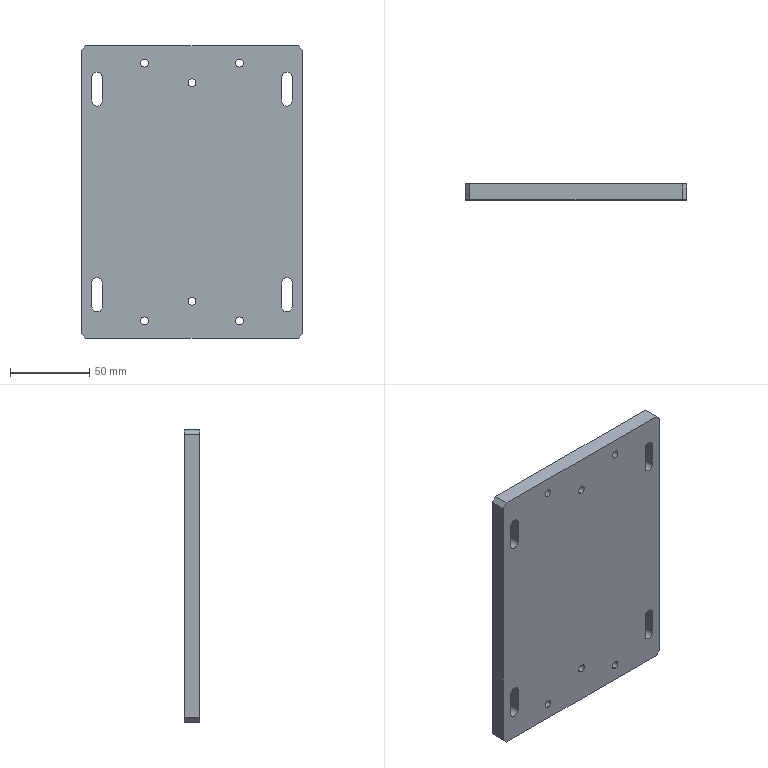Part | SolidWorks | features BaseBody 1 | 1 solid | 42 faces | box 140 x 10 x 185 mm | volume 252313 mm3 | cylinder 24 | plane 18 | commonest cylinder face diameters 5 x12 6.6 x12
STEP:
#1=CARTESIAN_POINT('',(0.,0.,-71.5));
#2=VERTEX_POINT('',#1);
#3=CARTESIAN_POINT('',(0.,10.,-71.5));
#4=VERTEX_POINT('',#3);
#5=CARTESIAN_POINT('',(0.,10.,-71.5));
#6=DIRECTION('',(0.,1.,0.));
#7=VECTOR('',#6,1000.);
#8=LINE('',#5,#7);
#9=EDGE_CURVE('',#2,#4,#8,.T.);
#10=ORIENTED_EDGE('',*,*,#9,.F.);
#11=CARTESIAN_POINT('',(0.,0.,-66.5));
#12=VERTEX_POINT('',#11);
#13=CARTESIAN_POINT('',(0.,0.,-69.));
#14=DIRECTION('',(0.,1.,0.));
#15=DIRECTION('',(0.,0.,1.));
#16=AXIS2_PLACEMENT_3D('',#13,#14,#15);
#17=CIRCLE('',#16,2.5);
#18=EDGE_CURVE('',#12,#2,#17,.T.);
#19=ORIENTED_EDGE('',*,*,#18,.F.);
#20=CARTESIAN_POINT('',(0.,10.,-66.5));
#21=VERTEX_POINT('',#20);
#22=CARTESIAN_POINT('',(0.,10.,-66.5));
#23=DIRECTION('',(0.,1.,0.));
#24=VECTOR('',#23,1000.);
#25=LINE('',#22,#24);
#26=EDGE_CURVE('',#12,#21,#25,.T.);
#27=ORIENTED_EDGE('',*,*,#26,.T.);
#28=CARTESIAN_POINT('',(0.,10.,-69.));
#29=DIRECTION('',(0.,1.,0.));
#30=DIRECTION('',(0.,0.,1.));
#31=AXIS2_PLACEMENT_3D('',#28,#29,#30);
#32=CIRCLE('',#31,2.5);
#33=EDGE_CURVE('',#21,#4,#32,.T.);
#34=ORIENTED_EDGE('',*,*,#33,.T.);
#35=EDGE_LOOP('',(#10,#19,#27,#34));
#36=FACE_OUTER_BOUND('',#35,.T.);
#37=CARTESIAN_POINT('',(0.,10.,-69.));
#38=DIRECTION('',(0.,1.,0.));
#39=DIRECTION('',(0.,0.,1.));
#40=AXIS2_PLACEMENT_3D('',#37,#38,#39);
#41=CYLINDRICAL_SURFACE('',#40,2.5);
#42=ADVANCED_FACE('',(#36),#41,.F.);
#43=CARTESIAN_POINT('',(0.,0.,66.5));
#44=VERTEX_POINT('',#43);
#45=CARTESIAN_POINT('',(0.,10.,66.5));
#46=VERTEX_POINT('',#45);
#47=CARTESIAN_POINT('',(0.,10.,66.5));
#48=DIRECTION('',(0.,1.,0.));
#49=VECTOR('',#48,1000.);
#50=LINE('',#47,#49);
#51=EDGE_CURVE('',#44,#46,#50,.T.);
#52=ORIENTED_EDGE('',*,*,#51,.F.);
#53=CARTESIAN_POINT('',(0.,0.,71.5));
#54=VERTEX_POINT('',#53);
#55=CARTESIAN_POINT('',(0.,0.,69.));
#56=DIRECTION('',(0.,1.,0.));
#57=DIRECTION('',(0.,0.,1.));
#58=AXIS2_PLACEMENT_3D('',#55,#56,#57);
#59=CIRCLE('',#58,2.5);
#60=EDGE_CURVE('',#54,#44,#59,.T.);
#61=ORIENTED_EDGE('',*,*,#60,.F.);
#62=CARTESIAN_POINT('',(0.,10.,71.5));
#63=VERTEX_POINT('',#62);
#64=CARTESIAN_POINT('',(0.,10.,71.5));
#65=DIRECTION('',(0.,1.,0.));
#66=VECTOR('',#65,1000.);
#67=LINE('',#64,#66);
#68=EDGE_CURVE('',#54,#63,#67,.T.);
#69=ORIENTED_EDGE('',*,*,#68,.T.);
#70=CARTESIAN_POINT('',(0.,10.,69.));
#71=DIRECTION('',(0.,1.,0.));
#72=DIRECTION('',(0.,0.,1.));
#73=AXIS2_PLACEMENT_3D('',#70,#71,#72);
#74=CIRCLE('',#73,2.5);
#75=EDGE_CURVE('',#63,#46,#74,.T.);
#76=ORIENTED_EDGE('',*,*,#75,.T.);
#77=EDGE_LOOP('',(#52,#61,#69,#76));
#78=FACE_OUTER_BOUND('',#77,.T.);
#79=CARTESIAN_POINT('',(0.,10.,69.));
#80=DIRECTION('',(0.,1.,0.));
#81=DIRECTION('',(0.,0.,1.));
#82=AXIS2_PLACEMENT_3D('',#79,#80,#81);
#83=CYLINDRICAL_SURFACE('',#82,2.5);
#84=ADVANCED_FACE('',(#78),#83,.F.);
#85=CARTESIAN_POINT('',(67.,10.,92.5));
#86=VERTEX_POINT('',#85);
#87=CARTESIAN_POINT('',(70.,10.,89.5));
#88=VERTEX_POINT('',#87);
#89=CARTESIAN_POINT('',(79.75,10.,79.75));
#90=DIRECTION('',(0.7071,0.,-0.7071));
#91=VECTOR('',#90,1000.);
#92=LINE('',#89,#91);
#93=EDGE_CURVE('',#86,#88,#92,.T.);
#94=ORIENTED_EDGE('',*,*,#93,.F.);
#95=CARTESIAN_POINT('',(67.,0.,92.5));
#96=VERTEX_POINT('',#95);
#97=CARTESIAN_POINT('',(67.,10.,92.5));
#98=DIRECTION('',(0.,1.,0.));
#99=VECTOR('',#98,1000.);
#100=LINE('',#97,#99);
#101=EDGE_CURVE('',#96,#86,#100,.T.);
#102=ORIENTED_EDGE('',*,*,#101,.F.);
#103=CARTESIAN_POINT('',(70.,0.,89.5));
#104=VERTEX_POINT('',#103);
#105=CARTESIAN_POINT('',(70.,0.,89.5));
#106=DIRECTION('',(-0.7071,0.,0.7071));
#107=VECTOR('',#106,1000.);
#108=LINE('',#105,#107);
#109=EDGE_CURVE('',#104,#96,#108,.T.);
#110=ORIENTED_EDGE('',*,*,#109,.F.);
#111=CARTESIAN_POINT('',(70.,10.,89.5));
#112=DIRECTION('',(0.,-1.,0.));
#113=VECTOR('',#112,1000.);
#114=LINE('',#111,#113);
#115=EDGE_CURVE('',#88,#104,#114,.T.);
#116=ORIENTED_EDGE('',*,*,#115,.F.);
#117=EDGE_LOOP('',(#94,#102,#110,#116));
#118=FACE_OUTER_BOUND('',#117,.T.);
#119=CARTESIAN_POINT('',(70.,10.,89.5));
#120=DIRECTION('',(-0.7071,0.,-0.7071));
#121=DIRECTION('',(-0.7071,0.,0.7071));
#122=AXIS2_PLACEMENT_3D('',#119,#120,#121);
#123=PLANE('',#122);
#124=ADVANCED_FACE('',(#118),#123,.F.);
#125=CARTESIAN_POINT('',(70.,10.,-89.5));
#126=VERTEX_POINT('',#125);
#127=CARTESIAN_POINT('',(67.,10.,-92.5));
#128=VERTEX_POINT('',#127);
#129=CARTESIAN_POINT('',(79.75,10.,-79.75));
#130=DIRECTION('',(-0.7071,0.,-0.7071));
#131=VECTOR('',#130,1000.);
#132=LINE('',#129,#131);
#133=EDGE_CURVE('',#126,#128,#132,.T.);
#134=ORIENTED_EDGE('',*,*,#133,.F.);
#135=CARTESIAN_POINT('',(70.,0.,-89.5));
#136=VERTEX_POINT('',#135);
#137=CARTESIAN_POINT('',(70.,10.,-89.5));
#138=DIRECTION('',(0.,1.,0.));
#139=VECTOR('',#138,1000.);
#140=LINE('',#137,#139);
#141=EDGE_CURVE('',#136,#126,#140,.T.);
#142=ORIENTED_EDGE('',*,*,#141,.F.);
#143=CARTESIAN_POINT('',(67.,0.,-92.5));
#144=VERTEX_POINT('',#143);
#145=CARTESIAN_POINT('',(67.,0.,-92.5));
#146=DIRECTION('',(0.7071,0.,0.7071));
#147=VECTOR('',#146,1000.);
#148=LINE('',#145,#147);
#149=EDGE_CURVE('',#144,#136,#148,.T.);
#150=ORIENTED_EDGE('',*,*,#149,.F.);
#151=CARTESIAN_POINT('',(67.,10.,-92.5));
#152=DIRECTION('',(0.,-1.,0.));
#153=VECTOR('',#152,1000.);
#154=LINE('',#151,#153);
#155=EDGE_CURVE('',#128,#144,#154,.T.);
#156=ORIENTED_EDGE('',*,*,#155,.F.);
#157=EDGE_LOOP('',(#134,#142,#150,#156));
#158=FACE_OUTER_BOUND('',#157,.T.);
#159=CARTESIAN_POINT('',(67.,10.,-92.5));
#160=DIRECTION('',(-0.7071,0.,0.7071));
#161=DIRECTION('',(0.,1.,0.));
#162=AXIS2_PLACEMENT_3D('',#159,#160,#161);
#163=PLANE('',#162);
#164=ADVANCED_FACE('',(#158),#163,.F.);
#165=CARTESIAN_POINT('',(-70.,10.,89.5));
#166=VERTEX_POINT('',#165);
#167=CARTESIAN_POINT('',(-67.,10.,92.5));
#168=VERTEX_POINT('',#167);
#169=CARTESIAN_POINT('',(-79.75,10.,79.75));
#170=DIRECTION('',(0.7071,0.,0.7071));
#171=VECTOR('',#170,1000.);
#172=LINE('',#169,#171);
#173=EDGE_CURVE('',#166,#168,#172,.T.);
#174=ORIENTED_EDGE('',*,*,#173,.F.);
#175=CARTESIAN_POINT('',(-70.,0.,89.5));
#176=VERTEX_POINT('',#175);
#177=CARTESIAN_POINT('',(-70.,10.,89.5));
#178=DIRECTION('',(0.,1.,0.));
#179=VECTOR('',#178,1000.);
#180=LINE('',#177,#179);
#181=EDGE_CURVE('',#176,#166,#180,.T.);
#182=ORIENTED_EDGE('',*,*,#181,.F.);
#183=CARTESIAN_POINT('',(-67.,0.,92.5));
#184=VERTEX_POINT('',#183);
#185=CARTESIAN_POINT('',(-67.,0.,92.5));
#186=DIRECTION('',(-0.7071,0.,-0.7071));
#187=VECTOR('',#186,1000.);
#188=LINE('',#185,#187);
#189=EDGE_CURVE('',#184,#176,#188,.T.);
#190=ORIENTED_EDGE('',*,*,#189,.F.);
#191=CARTESIAN_POINT('',(-67.,10.,92.5));
#192=DIRECTION('',(0.,-1.,0.));
#193=VECTOR('',#192,1000.);
#194=LINE('',#191,#193);
#195=EDGE_CURVE('',#168,#184,#194,.T.);
#196=ORIENTED_EDGE('',*,*,#195,.F.);
#197=EDGE_LOOP('',(#174,#182,#190,#196));
#198=FACE_OUTER_BOUND('',#197,.T.);
#199=CARTESIAN_POINT('',(-67.,10.,92.5));
#200=DIRECTION('',(0.7071,0.,-0.7071));
#201=DIRECTION('',(0.,-1.,0.));
#202=AXIS2_PLACEMENT_3D('',#199,#200,#201);
#203=PLANE('',#202);
#204=ADVANCED_FACE('',(#198),#203,.F.);
#205=CARTESIAN_POINT('',(-67.,10.,-92.5));
#206=VERTEX_POINT('',#205);
#207=CARTESIAN_POINT('',(-70.,10.,-89.5));
#208=VERTEX_POINT('',#207);
#209=CARTESIAN_POINT('',(-79.75,10.,-79.75));
#210=DIRECTION('',(-0.7071,0.,0.7071));
#211=VECTOR('',#210,1000.);
#212=LINE('',#209,#211);
#213=EDGE_CURVE('',#206,#208,#212,.T.);
#214=ORIENTED_EDGE('',*,*,#213,.F.);
#215=CARTESIAN_POINT('',(-67.,0.,-92.5));
#216=VERTEX_POINT('',#215);
#217=CARTESIAN_POINT('',(-67.,10.,-92.5));
#218=DIRECTION('',(0.,1.,0.));
#219=VECTOR('',#218,1000.);
#220=LINE('',#217,#219);
#221=EDGE_CURVE('',#216,#206,#220,.T.);
#222=ORIENTED_EDGE('',*,*,#221,.F.);
#223=CARTESIAN_POINT('',(-70.,0.,-89.5));
#224=VERTEX_POINT('',#223);
#225=CARTESIAN_POINT('',(-70.,0.,-89.5));
#226=DIRECTION('',(0.7071,0.,-0.7071));
#227=VECTOR('',#226,1000.);
#228=LINE('',#225,#227);
#229=EDGE_CURVE('',#224,#216,#228,.T.);
#230=ORIENTED_EDGE('',*,*,#229,.F.);
#231=CARTESIAN_POINT('',(-70.,10.,-89.5));
#232=DIRECTION('',(0.,-1.,0.));
#233=VECTOR('',#232,1000.);
#234=LINE('',#231,#233);
#235=EDGE_CURVE('',#208,#224,#234,.T.);
#236=ORIENTED_EDGE('',*,*,#235,.F.);
#237=EDGE_LOOP('',(#214,#222,#230,#236));
#238=FACE_OUTER_BOUND('',#237,.T.);
#239=CARTESIAN_POINT('',(-70.,10.,-89.5));
#240=DIRECTION('',(0.7071,0.,0.7071));
#241=DIRECTION('',(0.,-1.,0.));
#242=AXIS2_PLACEMENT_3D('',#239,#240,#241);
#243=PLANE('',#242);
#244=ADVANCED_FACE('',(#238),#243,.F.);
#245=CARTESIAN_POINT('',(63.3,10.,57.5));
#246=VERTEX_POINT('',#245);
#247=CARTESIAN_POINT('',(63.3,0.,57.5));
#248=VERTEX_POINT('',#247);
#249=CARTESIAN_POINT('',(63.3,0.,57.5));
#250=DIRECTION('',(0.,-1.,0.));
#251=VECTOR('',#250,1000.);
#252=LINE('',#249,#251);
#253=EDGE_CURVE('',#246,#248,#252,.T.);
#254=ORIENTED_EDGE('',*,*,#253,.T.);
#255=CARTESIAN_POINT('',(63.3,0.,72.5));
#256=VERTEX_POINT('',#255);
#257=CARTESIAN_POINT('',(63.3,0.,72.5));
#258=DIRECTION('',(0.,0.,-1.));
#259=VECTOR('',#258,1000.);
#260=LINE('',#257,#259);
#261=EDGE_CURVE('',#256,#248,#260,.T.);
#262=ORIENTED_EDGE('',*,*,#261,.F.);
#263=CARTESIAN_POINT('',(63.3,10.,72.5));
#264=VERTEX_POINT('',#263);
#265=CARTESIAN_POINT('',(63.3,0.,72.5));
#266=DIRECTION('',(0.,-1.,0.));
#267=VECTOR('',#266,1000.);
#268=LINE('',#265,#267);
#269=EDGE_CURVE('',#264,#256,#268,.T.);
#270=ORIENTED_EDGE('',*,*,#269,.F.);
#271=CARTESIAN_POINT('',(63.3,10.,72.5));
#272=DIRECTION('',(0.,0.,-1.));
#273=VECTOR('',#272,1000.);
#274=LINE('',#271,#273);
#275=EDGE_CURVE('',#264,#246,#274,.T.);
#276=ORIENTED_EDGE('',*,*,#275,.T.);
#277=EDGE_LOOP('',(#254,#262,#270,#276));
#278=FACE_OUTER_BOUND('',#277,.T.);
#279=CARTESIAN_POINT('',(63.3,0.,72.5));
#280=DIRECTION('',(1.,0.,0.));
#281=DIRECTION('',(0.,-1.,0.));
#282=AXIS2_PLACEMENT_3D('',#279,#280,#281);
#283=PLANE('',#282);
#284=ADVANCED_FACE('',(#278),#283,.F.);
#285=CARTESIAN_POINT('',(56.7,0.,57.5));
#286=VERTEX_POINT('',#285);
#287=CARTESIAN_POINT('',(56.7,10.,57.5));
#288=VERTEX_POINT('',#287);
#289=CARTESIAN_POINT('',(56.7,10.,57.5));
#290=DIRECTION('',(0.,1.,0.));
#291=VECTOR('',#290,1000.);
#292=LINE('',#289,#291);
#293=EDGE_CURVE('',#286,#288,#292,.T.);
#294=ORIENTED_EDGE('',*,*,#293,.T.);
#295=CARTESIAN_POINT('',(56.7,10.,72.5));
#296=VERTEX_POINT('',#295);
#297=CARTESIAN_POINT('',(56.7,10.,72.5));
#298=DIRECTION('',(0.,0.,-1.));
#299=VECTOR('',#298,1000.);
#300=LINE('',#297,#299);
#301=EDGE_CURVE('',#296,#288,#300,.T.);
#302=ORIENTED_EDGE('',*,*,#301,.F.);
#303=CARTESIAN_POINT('',(56.7,0.,72.5));
#304=VERTEX_POINT('',#303);
#305=CARTESIAN_POINT('',(56.7,10.,72.5));
#306=DIRECTION('',(0.,-1.,0.));
#307=VECTOR('',#306,1000.);
#308=LINE('',#305,#307);
#309=EDGE_CURVE('',#296,#304,#308,.T.);
#310=ORIENTED_EDGE('',*,*,#309,.T.);
#311=CARTESIAN_POINT('',(56.7,0.,72.5));
#312=DIRECTION('',(0.,0.,-1.));
#313=VECTOR('',#312,1000.);
#314=LINE('',#311,#313);
#315=EDGE_CURVE('',#304,#286,#314,.T.);
#316=ORIENTED_EDGE('',*,*,#315,.T.);
#317=EDGE_LOOP('',(#294,#302,#310,#316));
#318=FACE_OUTER_BOUND('',#317,.T.);
#319=CARTESIAN_POINT('',(56.7,10.,72.5));
#320=DIRECTION('',(-1.,0.,0.));
#321=DIRECTION('',(0.,0.,1.));
#322=AXIS2_PLACEMENT_3D('',#319,#320,#321);
#323=PLANE('',#322);
#324=ADVANCED_FACE('',(#318),#323,.F.);
#325=CARTESIAN_POINT('',(60.,0.,75.8));
#326=VERTEX_POINT('',#325);
#327=CARTESIAN_POINT('',(60.,10.,75.8));
#328=VERTEX_POINT('',#327);
#329=CARTESIAN_POINT('',(60.,10.,75.8));
#330=DIRECTION('',(0.,1.,0.));
#331=VECTOR('',#330,1000.);
#332=LINE('',#329,#331);
#333=EDGE_CURVE('',#326,#328,#332,.T.);
#334=ORIENTED_EDGE('',*,*,#333,.F.);
#335=CARTESIAN_POINT('',(60.,0.,72.5));
#336=DIRECTION('',(0.,1.,0.));
#337=DIRECTION('',(0.,0.,1.));
#338=AXIS2_PLACEMENT_3D('',#335,#336,#337);
#339=CIRCLE('',#338,3.3);
#340=EDGE_CURVE('',#304,#326,#339,.T.);
#341=ORIENTED_EDGE('',*,*,#340,.F.);
#342=ORIENTED_EDGE('',*,*,#309,.F.);
#343=CARTESIAN_POINT('',(60.,10.,72.5));
#344=DIRECTION('',(0.,1.,0.));
#345=DIRECTION('',(0.,0.,1.));
#346=AXIS2_PLACEMENT_3D('',#343,#344,#345);
#347=CIRCLE('',#346,3.3);
#348=EDGE_CURVE('',#296,#328,#347,.T.);
#349=ORIENTED_EDGE('',*,*,#348,.T.);
#350=EDGE_LOOP('',(#334,#341,#342,#349));
#351=FACE_OUTER_BOUND('',#350,.T.);
#352=CARTESIAN_POINT('',(60.,10.,72.5));
#353=DIRECTION('',(0.,1.,0.));
#354=DIRECTION('',(0.,0.,1.));
#355=AXIS2_PLACEMENT_3D('',#352,#353,#354);
#356=CYLINDRICAL_SURFACE('',#355,3.3);
#357=ADVANCED_FACE('',(#351),#356,.F.);
#358=CARTESIAN_POINT('',(60.,0.,57.5));
#359=DIRECTION('',(0.,1.,0.));
#360=DIRECTION('',(0.,0.,1.));
#361=AXIS2_PLACEMENT_3D('',#358,#359,#360);
#362=CIRCLE('',#361,3.3);
#363=EDGE_CURVE('',#248,#286,#362,.T.);
#364=ORIENTED_EDGE('',*,*,#363,.F.);
#365=ORIENTED_EDGE('',*,*,#253,.F.);
#366=CARTESIAN_POINT('',(60.,10.,57.5));
#367=DIRECTION('',(0.,1.,0.));
#368=DIRECTION('',(0.,0.,1.));
#369=AXIS2_PLACEMENT_3D('',#366,#367,#368);
#370=CIRCLE('',#369,3.3);
#371=EDGE_CURVE('',#246,#288,#370,.T.);
#372=ORIENTED_EDGE('',*,*,#371,.T.);
#373=ORIENTED_EDGE('',*,*,#293,.F.);
#374=EDGE_LOOP('',(#364,#365,#372,#373));
#375=FACE_OUTER_BOUND('',#374,.T.);
#376=CARTESIAN_POINT('',(60.,10.,57.5));
#377=DIRECTION('',(0.,1.,0.));
#378=DIRECTION('',(0.,0.,1.));
#379=AXIS2_PLACEMENT_3D('',#376,#377,#378);
#380=CYLINDRICAL_SURFACE('',#379,3.3);
#381=ADVANCED_FACE('',(#375),#380,.F.);
#382=CARTESIAN_POINT('',(63.3,10.,-72.5));
#383=VERTEX_POINT('',#382);
#384=CARTESIAN_POINT('',(63.3,0.,-72.5));
#385=VERTEX_POINT('',#384);
#386=CARTESIAN_POINT('',(63.3,0.,-72.5));
#387=DIRECTION('',(0.,-1.,0.));
#388=VECTOR('',#387,1000.);
#389=LINE('',#386,#388);
#390=EDGE_CURVE('',#383,#385,#389,.T.);
#391=ORIENTED_EDGE('',*,*,#390,.T.);
#392=CARTESIAN_POINT('',(63.3,0.,-57.5));
#393=VERTEX_POINT('',#392);
#394=CARTESIAN_POINT('',(63.3,0.,-57.5));
#395=DIRECTION('',(0.,0.,-1.));
#396=VECTOR('',#395,1000.);
#397=LINE('',#394,#396);
#398=EDGE_CURVE('',#393,#385,#397,.T.);
#399=ORIENTED_EDGE('',*,*,#398,.F.);
#400=CARTESIAN_POINT('',(63.3,10.,-57.5));
#401=VERTEX_POINT('',#400);
#402=CARTESIAN_POINT('',(63.3,0.,-57.5));
#403=DIRECTION('',(0.,-1.,0.));
#404=VECTOR('',#403,1000.);
#405=LINE('',#402,#404);
#406=EDGE_CURVE('',#401,#393,#405,.T.);
#407=ORIENTED_EDGE('',*,*,#406,.F.);
#408=CARTESIAN_POINT('',(63.3,10.,-57.5));
#409=DIRECTION('',(0.,0.,-1.));
#410=VECTOR('',#409,1000.);
#411=LINE('',#408,#410);
#412=EDGE_CURVE('',#401,#383,#411,.T.);
#413=ORIENTED_EDGE('',*,*,#412,.T.);
#414=EDGE_LOOP('',(#391,#399,#407,#413));
#415=FACE_OUTER_BOUND('',#414,.T.);
#416=CARTESIAN_POINT('',(63.3,0.,-57.5));
#417=DIRECTION('',(1.,0.,0.));
#418=DIRECTION('',(0.,-1.,0.));
#419=AXIS2_PLACEMENT_3D('',#416,#417,#418);
#420=PLANE('',#419);
#421=ADVANCED_FACE('',(#415),#420,.F.);
#422=CARTESIAN_POINT('',(56.7,0.,-72.5));
#423=VERTEX_POINT('',#422);
#424=CARTESIAN_POINT('',(56.7,10.,-72.5));
#425=VERTEX_POINT('',#424);
#426=CARTESIAN_POINT('',(56.7,10.,-72.5));
#427=DIRECTION('',(0.,1.,0.));
#428=VECTOR('',#427,1000.);
#429=LINE('',#426,#428);
#430=EDGE_CURVE('',#423,#425,#429,.T.);
#431=ORIENTED_EDGE('',*,*,#430,.T.);
#432=CARTESIAN_POINT('',(56.7,10.,-57.5));
#433=VERTEX_POINT('',#432);
#434=CARTESIAN_POINT('',(56.7,10.,-57.5));
#435=DIRECTION('',(0.,0.,-1.));
#436=VECTOR('',#435,1000.);
#437=LINE('',#434,#436);
#438=EDGE_CURVE('',#433,#425,#437,.T.);
#439=ORIENTED_EDGE('',*,*,#438,.F.);
#440=CARTESIAN_POINT('',(56.7,0.,-57.5));
#441=VERTEX_POINT('',#440);
#442=CARTESIAN_POINT('',(56.7,10.,-57.5));
#443=DIRECTION('',(0.,-1.,0.));
#444=VECTOR('',#443,1000.);
#445=LINE('',#442,#444);
#446=EDGE_CURVE('',#433,#441,#445,.T.);
#447=ORIENTED_EDGE('',*,*,#446,.T.);
#448=CARTESIAN_POINT('',(56.7,0.,-57.5));
#449=DIRECTION('',(0.,0.,-1.));
#450=VECTOR('',#449,1000.);
#451=LINE('',#448,#450);
#452=EDGE_CURVE('',#441,#423,#451,.T.);
#453=ORIENTED_EDGE('',*,*,#452,.T.);
#454=EDGE_LOOP('',(#431,#439,#447,#453));
#455=FACE_OUTER_BOUND('',#454,.T.);
#456=CARTESIAN_POINT('',(56.7,10.,-57.5));
#457=DIRECTION('',(-1.,0.,0.));
#458=DIRECTION('',(0.,0.,1.));
#459=AXIS2_PLACEMENT_3D('',#456,#457,#458);
#460=PLANE('',#459);
#461=ADVANCED_FACE('',(#455),#460,.F.);
#462=CARTESIAN_POINT('',(60.,0.,-54.2));
#463=VERTEX_POINT('',#462);
#464=CARTESIAN_POINT('',(60.,10.,-54.2));
#465=VERTEX_POINT('',#464);
#466=CARTESIAN_POINT('',(60.,10.,-54.2));
#467=DIRECTION('',(0.,1.,0.));
#468=VECTOR('',#467,1000.);
#469=LINE('',#466,#468);
#470=EDGE_CURVE('',#463,#465,#469,.T.);
#471=ORIENTED_EDGE('',*,*,#470,.F.);
#472=CARTESIAN_POINT('',(60.,0.,-57.5));
#473=DIRECTION('',(0.,1.,0.));
#474=DIRECTION('',(0.,0.,1.));
#475=AXIS2_PLACEMENT_3D('',#472,#473,#474);
#476=CIRCLE('',#475,3.3);
#477=EDGE_CURVE('',#441,#463,#476,.T.);
#478=ORIENTED_EDGE('',*,*,#477,.F.);
#479=ORIENTED_EDGE('',*,*,#446,.F.);
#480=CARTESIAN_POINT('',(60.,10.,-57.5));
#481=DIRECTION('',(0.,1.,0.));
#482=DIRECTION('',(0.,0.,1.));
#483=AXIS2_PLACEMENT_3D('',#480,#481,#482);
#484=CIRCLE('',#483,3.3);
#485=EDGE_CURVE('',#433,#465,#484,.T.);
#486=ORIENTED_EDGE('',*,*,#485,.T.);
#487=EDGE_LOOP('',(#471,#478,#479,#486));
#488=FACE_OUTER_BOUND('',#487,.T.);
#489=CARTESIAN_POINT('',(60.,10.,-57.5));
#490=DIRECTION('',(0.,1.,0.));
#491=DIRECTION('',(0.,0.,1.));
#492=AXIS2_PLACEMENT_3D('',#489,#490,#491);
#493=CYLINDRICAL_SURFACE('',#492,3.3);
#494=ADVANCED_FACE('',(#488),#493,.F.);
#495=CARTESIAN_POINT('',(60.,0.,-72.5));
#496=DIRECTION('',(0.,1.,0.));
#497=DIRECTION('',(0.,0.,1.));
#498=AXIS2_PLACEMENT_3D('',#495,#496,#497);
#499=CIRCLE('',#498,3.3);
#500=EDGE_CURVE('',#385,#423,#499,.T.);
#501=ORIENTED_EDGE('',*,*,#500,.F.);
#502=ORIENTED_EDGE('',*,*,#390,.F.);
#503=CARTESIAN_POINT('',(60.,10.,-72.5));
#504=DIRECTION('',(0.,1.,0.));
#505=DIRECTION('',(0.,0.,1.));
#506=AXIS2_PLACEMENT_3D('',#503,#504,#505);
#507=CIRCLE('',#506,3.3);
#508=EDGE_CURVE('',#383,#425,#507,.T.);
#509=ORIENTED_EDGE('',*,*,#508,.T.);
#510=ORIENTED_EDGE('',*,*,#430,.F.);
#511=EDGE_LOOP('',(#501,#502,#509,#510));
#512=FACE_OUTER_BOUND('',#511,.T.);
#513=CARTESIAN_POINT('',(60.,10.,-72.5));
#514=DIRECTION('',(0.,1.,0.));
#515=DIRECTION('',(0.,0.,1.));
#516=AXIS2_PLACEMENT_3D('',#513,#514,#515);
#517=CYLINDRICAL_SURFACE('',#516,3.3);
#518=ADVANCED_FACE('',(#512),#517,.F.);
#519=CARTESIAN_POINT('',(-56.7,10.,-72.5));
#520=VERTEX_POINT('',#519);
#521=CARTESIAN_POINT('',(-56.7,0.,-72.5));
#522=VERTEX_POINT('',#521);
#523=CARTESIAN_POINT('',(-56.7,0.,-72.5));
#524=DIRECTION('',(0.,-1.,0.));
#525=VECTOR('',#524,1000.);
#526=LINE('',#523,#525);
#527=EDGE_CURVE('',#520,#522,#526,.T.);
#528=ORIENTED_EDGE('',*,*,#527,.T.);
#529=CARTESIAN_POINT('',(-56.7,0.,-57.5));
#530=VERTEX_POINT('',#529);
#531=CARTESIAN_POINT('',(-56.7,0.,-57.5));
#532=DIRECTION('',(0.,0.,-1.));
#533=VECTOR('',#532,1000.);
#534=LINE('',#531,#533);
#535=EDGE_CURVE('',#530,#522,#534,.T.);
#536=ORIENTED_EDGE('',*,*,#535,.F.);
#537=CARTESIAN_POINT('',(-56.7,10.,-57.5));
#538=VERTEX_POINT('',#537);
#539=CARTESIAN_POINT('',(-56.7,0.,-57.5));
#540=DIRECTION('',(0.,-1.,0.));
#541=VECTOR('',#540,1000.);
#542=LINE('',#539,#541);
#543=EDGE_CURVE('',#538,#530,#542,.T.);
#544=ORIENTED_EDGE('',*,*,#543,.F.);
#545=CARTESIAN_POINT('',(-56.7,10.,-57.5));
#546=DIRECTION('',(0.,0.,-1.));
#547=VECTOR('',#546,1000.);
#548=LINE('',#545,#547);
#549=EDGE_CURVE('',#538,#520,#548,.T.);
#550=ORIENTED_EDGE('',*,*,#549,.T.);
#551=EDGE_LOOP('',(#528,#536,#544,#550));
#552=FACE_OUTER_BOUND('',#551,.T.);
#553=CARTESIAN_POINT('',(-56.7,0.,-57.5));
#554=DIRECTION('',(1.,0.,0.));
#555=DIRECTION('',(0.,-1.,0.));
#556=AXIS2_PLACEMENT_3D('',#553,#554,#555);
#557=PLANE('',#556);
#558=ADVANCED_FACE('',(#552),#557,.F.);
#559=CARTESIAN_POINT('',(-63.3,0.,-72.5));
#560=VERTEX_POINT('',#559);
#561=CARTESIAN_POINT('',(-63.3,10.,-72.5));
#562=VERTEX_POINT('',#561);
#563=CARTESIAN_POINT('',(-63.3,10.,-72.5));
#564=DIRECTION('',(0.,1.,0.));
#565=VECTOR('',#564,1000.);
#566=LINE('',#563,#565);
#567=EDGE_CURVE('',#560,#562,#566,.T.);
#568=ORIENTED_EDGE('',*,*,#567,.T.);
#569=CARTESIAN_POINT('',(-63.3,10.,-57.5));
#570=VERTEX_POINT('',#569);
#571=CARTESIAN_POINT('',(-63.3,10.,-57.5));
#572=DIRECTION('',(0.,0.,-1.));
#573=VECTOR('',#572,1000.);
#574=LINE('',#571,#573);
#575=EDGE_CURVE('',#570,#562,#574,.T.);
#576=ORIENTED_EDGE('',*,*,#575,.F.);
#577=CARTESIAN_POINT('',(-63.3,0.,-57.5));
#578=VERTEX_POINT('',#577);
#579=CARTESIAN_POINT('',(-63.3,10.,-57.5));
#580=DIRECTION('',(0.,-1.,0.));
#581=VECTOR('',#580,1000.);
#582=LINE('',#579,#581);
#583=EDGE_CURVE('',#570,#578,#582,.T.);
#584=ORIENTED_EDGE('',*,*,#583,.T.);
#585=CARTESIAN_POINT('',(-63.3,0.,-57.5));
#586=DIRECTION('',(0.,0.,-1.));
#587=VECTOR('',#586,1000.);
#588=LINE('',#585,#587);
#589=EDGE_CURVE('',#578,#560,#588,.T.);
#590=ORIENTED_EDGE('',*,*,#589,.T.);
#591=EDGE_LOOP('',(#568,#576,#584,#590));
#592=FACE_OUTER_BOUND('',#591,.T.);
#593=CARTESIAN_POINT('',(-63.3,10.,-57.5));
#594=DIRECTION('',(-1.,0.,0.));
#595=DIRECTION('',(0.,0.,1.));
#596=AXIS2_PLACEMENT_3D('',#593,#594,#595);
#597=PLANE('',#596);
#598=ADVANCED_FACE('',(#592),#597,.F.);
#599=CARTESIAN_POINT('',(-60.,0.,-54.2));
#600=VERTEX_POINT('',#599);
#601=CARTESIAN_POINT('',(-60.,10.,-54.2));
#602=VERTEX_POINT('',#601);
#603=CARTESIAN_POINT('',(-60.,10.,-54.2));
#604=DIRECTION('',(0.,1.,0.));
#605=VECTOR('',#604,1000.);
#606=LINE('',#603,#605);
#607=EDGE_CURVE('',#600,#602,#606,.T.);
#608=ORIENTED_EDGE('',*,*,#607,.F.);
#609=CARTESIAN_POINT('',(-60.,0.,-57.5));
#610=DIRECTION('',(0.,1.,0.));
#611=DIRECTION('',(0.,0.,1.));
#612=AXIS2_PLACEMENT_3D('',#609,#610,#611);
#613=CIRCLE('',#612,3.3);
#614=EDGE_CURVE('',#578,#600,#613,.T.);
#615=ORIENTED_EDGE('',*,*,#614,.F.);
#616=ORIENTED_EDGE('',*,*,#583,.F.);
#617=CARTESIAN_POINT('',(-60.,10.,-57.5));
#618=DIRECTION('',(0.,1.,0.));
#619=DIRECTION('',(0.,0.,1.));
#620=AXIS2_PLACEMENT_3D('',#617,#618,#619);
#621=CIRCLE('',#620,3.3);
#622=EDGE_CURVE('',#570,#602,#621,.T.);
#623=ORIENTED_EDGE('',*,*,#622,.T.);
#624=EDGE_LOOP('',(#608,#615,#616,#623));
#625=FACE_OUTER_BOUND('',#624,.T.);
#626=CARTESIAN_POINT('',(-60.,10.,-57.5));
#627=DIRECTION('',(0.,1.,0.));
#628=DIRECTION('',(0.,0.,1.));
#629=AXIS2_PLACEMENT_3D('',#626,#627,#628);
#630=CYLINDRICAL_SURFACE('',#629,3.3);
#631=ADVANCED_FACE('',(#625),#630,.F.);
#632=CARTESIAN_POINT('',(-60.,0.,-72.5));
#633=DIRECTION('',(0.,1.,0.));
#634=DIRECTION('',(0.,0.,1.));
#635=AXIS2_PLACEMENT_3D('',#632,#633,#634);
#636=CIRCLE('',#635,3.3);
#637=EDGE_CURVE('',#522,#560,#636,.T.);
#638=ORIENTED_EDGE('',*,*,#637,.F.);
#639=ORIENTED_EDGE('',*,*,#527,.F.);
#640=CARTESIAN_POINT('',(-60.,10.,-72.5));
#641=DIRECTION('',(0.,1.,0.));
#642=DIRECTION('',(0.,0.,1.));
#643=AXIS2_PLACEMENT_3D('',#640,#641,#642);
#644=CIRCLE('',#643,3.3);
#645=EDGE_CURVE('',#520,#562,#644,.T.);
#646=ORIENTED_EDGE('',*,*,#645,.T.);
#647=ORIENTED_EDGE('',*,*,#567,.F.);
#648=EDGE_LOOP('',(#638,#639,#646,#647));
#649=FACE_OUTER_BOUND('',#648,.T.);
#650=CARTESIAN_POINT('',(-60.,10.,-72.5));
#651=DIRECTION('',(0.,1.,0.));
#652=DIRECTION('',(0.,0.,1.));
#653=AXIS2_PLACEMENT_3D('',#650,#651,#652);
#654=CYLINDRICAL_SURFACE('',#653,3.3);
#655=ADVANCED_FACE('',(#649),#654,.F.);
#656=CARTESIAN_POINT('',(-56.7,10.,57.5));
#657=VERTEX_POINT('',#656);
#658=CARTESIAN_POINT('',(-56.7,0.,57.5));
#659=VERTEX_POINT('',#658);
#660=CARTESIAN_POINT('',(-56.7,0.,57.5));
#661=DIRECTION('',(0.,-1.,0.));
#662=VECTOR('',#661,1000.);
#663=LINE('',#660,#662);
#664=EDGE_CURVE('',#657,#659,#663,.T.);
#665=ORIENTED_EDGE('',*,*,#664,.T.);
#666=CARTESIAN_POINT('',(-56.7,0.,72.5));
#667=VERTEX_POINT('',#666);
#668=CARTESIAN_POINT('',(-56.7,0.,72.5));
#669=DIRECTION('',(0.,0.,-1.));
#670=VECTOR('',#669,1000.);
#671=LINE('',#668,#670);
#672=EDGE_CURVE('',#667,#659,#671,.T.);
#673=ORIENTED_EDGE('',*,*,#672,.F.);
#674=CARTESIAN_POINT('',(-56.7,10.,72.5));
#675=VERTEX_POINT('',#674);
#676=CARTESIAN_POINT('',(-56.7,0.,72.5));
#677=DIRECTION('',(0.,-1.,0.));
#678=VECTOR('',#677,1000.);
#679=LINE('',#676,#678);
#680=EDGE_CURVE('',#675,#667,#679,.T.);
#681=ORIENTED_EDGE('',*,*,#680,.F.);
#682=CARTESIAN_POINT('',(-56.7,10.,72.5));
#683=DIRECTION('',(0.,0.,-1.));
#684=VECTOR('',#683,1000.);
#685=LINE('',#682,#684);
#686=EDGE_CURVE('',#675,#657,#685,.T.);
#687=ORIENTED_EDGE('',*,*,#686,.T.);
#688=EDGE_LOOP('',(#665,#673,#681,#687));
#689=FACE_OUTER_BOUND('',#688,.T.);
#690=CARTESIAN_POINT('',(-56.7,0.,72.5));
#691=DIRECTION('',(1.,0.,0.));
#692=DIRECTION('',(0.,-1.,0.));
#693=AXIS2_PLACEMENT_3D('',#690,#691,#692);
#694=PLANE('',#693);
#695=ADVANCED_FACE('',(#689),#694,.F.);
#696=CARTESIAN_POINT('',(-63.3,0.,57.5));
#697=VERTEX_POINT('',#696);
#698=CARTESIAN_POINT('',(-63.3,10.,57.5));
#699=VERTEX_POINT('',#698);
#700=CARTESIAN_POINT('',(-63.3,10.,57.5));
#701=DIRECTION('',(0.,1.,0.));
#702=VECTOR('',#701,1000.);
#703=LINE('',#700,#702);
#704=EDGE_CURVE('',#697,#699,#703,.T.);
#705=ORIENTED_EDGE('',*,*,#704,.T.);
#706=CARTESIAN_POINT('',(-63.3,10.,72.5));
#707=VERTEX_POINT('',#706);
#708=CARTESIAN_POINT('',(-63.3,10.,72.5));
#709=DIRECTION('',(0.,0.,-1.));
#710=VECTOR('',#709,1000.);
#711=LINE('',#708,#710);
#712=EDGE_CURVE('',#707,#699,#711,.T.);
#713=ORIENTED_EDGE('',*,*,#712,.F.);
#714=CARTESIAN_POINT('',(-63.3,0.,72.5));
#715=VERTEX_POINT('',#714);
#716=CARTESIAN_POINT('',(-63.3,10.,72.5));
#717=DIRECTION('',(0.,-1.,0.));
#718=VECTOR('',#717,1000.);
#719=LINE('',#716,#718);
#720=EDGE_CURVE('',#707,#715,#719,.T.);
#721=ORIENTED_EDGE('',*,*,#720,.T.);
#722=CARTESIAN_POINT('',(-63.3,0.,72.5));
#723=DIRECTION('',(0.,0.,-1.));
#724=VECTOR('',#723,1000.);
#725=LINE('',#722,#724);
#726=EDGE_CURVE('',#715,#697,#725,.T.);
#727=ORIENTED_EDGE('',*,*,#726,.T.);
#728=EDGE_LOOP('',(#705,#713,#721,#727));
#729=FACE_OUTER_BOUND('',#728,.T.);
#730=CARTESIAN_POINT('',(-63.3,10.,72.5));
#731=DIRECTION('',(-1.,0.,0.));
#732=DIRECTION('',(0.,0.,1.));
#733=AXIS2_PLACEMENT_3D('',#730,#731,#732);
#734=PLANE('',#733);
#735=ADVANCED_FACE('',(#729),#734,.F.);
#736=CARTESIAN_POINT('',(-60.,0.,75.8));
#737=VERTEX_POINT('',#736);
#738=CARTESIAN_POINT('',(-60.,10.,75.8));
#739=VERTEX_POINT('',#738);
#740=CARTESIAN_POINT('',(-60.,10.,75.8));
#741=DIRECTION('',(0.,1.,0.));
#742=VECTOR('',#741,1000.);
#743=LINE('',#740,#742);
#744=EDGE_CURVE('',#737,#739,#743,.T.);
#745=ORIENTED_EDGE('',*,*,#744,.F.);
#746=CARTESIAN_POINT('',(-60.,0.,72.5));
#747=DIRECTION('',(0.,1.,0.));
#748=DIRECTION('',(0.,0.,1.));
#749=AXIS2_PLACEMENT_3D('',#746,#747,#748);
#750=CIRCLE('',#749,3.3);
#751=EDGE_CURVE('',#715,#737,#750,.T.);
#752=ORIENTED_EDGE('',*,*,#751,.F.);
#753=ORIENTED_EDGE('',*,*,#720,.F.);
#754=CARTESIAN_POINT('',(-60.,10.,72.5));
#755=DIRECTION('',(0.,1.,0.));
#756=DIRECTION('',(0.,0.,1.));
#757=AXIS2_PLACEMENT_3D('',#754,#755,#756);
#758=CIRCLE('',#757,3.3);
#759=EDGE_CURVE('',#707,#739,#758,.T.);
#760=ORIENTED_EDGE('',*,*,#759,.T.);
#761=EDGE_LOOP('',(#745,#752,#753,#760));
#762=FACE_OUTER_BOUND('',#761,.T.);
#763=CARTESIAN_POINT('',(-60.,10.,72.5));
#764=DIRECTION('',(0.,1.,0.));
#765=DIRECTION('',(0.,0.,1.));
#766=AXIS2_PLACEMENT_3D('',#763,#764,#765);
#767=CYLINDRICAL_SURFACE('',#766,3.3);
#768=ADVANCED_FACE('',(#762),#767,.F.);
#769=CARTESIAN_POINT('',(-60.,0.,57.5));
#770=DIRECTION('',(0.,1.,0.));
#771=DIRECTION('',(0.,0.,1.));
#772=AXIS2_PLACEMENT_3D('',#769,#770,#771);
#773=CIRCLE('',#772,3.3);
#774=EDGE_CURVE('',#659,#697,#773,.T.);
#775=ORIENTED_EDGE('',*,*,#774,.F.);
#776=ORIENTED_EDGE('',*,*,#664,.F.);
#777=CARTESIAN_POINT('',(-60.,10.,57.5));
#778=DIRECTION('',(0.,1.,0.));
#779=DIRECTION('',(0.,0.,1.));
#780=AXIS2_PLACEMENT_3D('',#777,#778,#779);
#781=CIRCLE('',#780,3.3);
#782=EDGE_CURVE('',#657,#699,#781,.T.);
#783=ORIENTED_EDGE('',*,*,#782,.T.);
#784=ORIENTED_EDGE('',*,*,#704,.F.);
#785=EDGE_LOOP('',(#775,#776,#783,#784));
#786=FACE_OUTER_BOUND('',#785,.T.);
#787=CARTESIAN_POINT('',(-60.,10.,57.5));
#788=DIRECTION('',(0.,1.,0.));
#789=DIRECTION('',(0.,0.,1.));
#790=AXIS2_PLACEMENT_3D('',#787,#788,#789);
#791=CYLINDRICAL_SURFACE('',#790,3.3);
#792=ADVANCED_FACE('',(#786),#791,.F.);
#793=CARTESIAN_POINT('',(-30.,0.,79.));
#794=VERTEX_POINT('',#793);
#795=CARTESIAN_POINT('',(-30.,10.,79.));
#796=VERTEX_POINT('',#795);
#797=CARTESIAN_POINT('',(-30.,10.,79.));
#798=DIRECTION('',(0.,1.,0.));
#799=VECTOR('',#798,1000.);
#800=LINE('',#797,#799);
#801=EDGE_CURVE('',#794,#796,#800,.T.);
#802=ORIENTED_EDGE('',*,*,#801,.F.);
#803=CARTESIAN_POINT('',(-30.,0.,84.));
#804=VERTEX_POINT('',#803);
#805=CARTESIAN_POINT('',(-30.,0.,81.5));
#806=DIRECTION('',(0.,1.,0.));
#807=DIRECTION('',(0.,0.,1.));
#808=AXIS2_PLACEMENT_3D('',#805,#806,#807);
#809=CIRCLE('',#808,2.5);
#810=EDGE_CURVE('',#804,#794,#809,.T.);
#811=ORIENTED_EDGE('',*,*,#810,.F.);
#812=CARTESIAN_POINT('',(-30.,10.,84.));
#813=VERTEX_POINT('',#812);
#814=CARTESIAN_POINT('',(-30.,10.,84.));
#815=DIRECTION('',(0.,1.,0.));
#816=VECTOR('',#815,1000.);
#817=LINE('',#814,#816);
#818=EDGE_CURVE('',#804,#813,#817,.T.);
#819=ORIENTED_EDGE('',*,*,#818,.T.);
#820=CARTESIAN_POINT('',(-30.,10.,81.5));
#821=DIRECTION('',(0.,1.,0.));
#822=DIRECTION('',(0.,0.,1.));
#823=AXIS2_PLACEMENT_3D('',#820,#821,#822);
#824=CIRCLE('',#823,2.5);
#825=EDGE_CURVE('',#813,#796,#824,.T.);
#826=ORIENTED_EDGE('',*,*,#825,.T.);
#827=EDGE_LOOP('',(#802,#811,#819,#826));
#828=FACE_OUTER_BOUND('',#827,.T.);
#829=CARTESIAN_POINT('',(-30.,10.,81.5));
#830=DIRECTION('',(0.,1.,0.));
#831=DIRECTION('',(0.,0.,1.));
#832=AXIS2_PLACEMENT_3D('',#829,#830,#831);
#833=CYLINDRICAL_SURFACE('',#832,2.5);
#834=ADVANCED_FACE('',(#828),#833,.F.);
#835=CARTESIAN_POINT('',(-30.,0.,-84.));
#836=VERTEX_POINT('',#835);
#837=CARTESIAN_POINT('',(-30.,10.,-84.));
#838=VERTEX_POINT('',#837);
#839=CARTESIAN_POINT('',(-30.,10.,-84.));
#840=DIRECTION('',(0.,1.,0.));
#841=VECTOR('',#840,1000.);
#842=LINE('',#839,#841);
#843=EDGE_CURVE('',#836,#838,#842,.T.);
#844=ORIENTED_EDGE('',*,*,#843,.F.);
#845=CARTESIAN_POINT('',(-30.,0.,-79.));
#846=VERTEX_POINT('',#845);
#847=CARTESIAN_POINT('',(-30.,0.,-81.5));
#848=DIRECTION('',(0.,1.,0.));
#849=DIRECTION('',(0.,0.,1.));
#850=AXIS2_PLACEMENT_3D('',#847,#848,#849);
#851=CIRCLE('',#850,2.5);
#852=EDGE_CURVE('',#846,#836,#851,.T.);
#853=ORIENTED_EDGE('',*,*,#852,.F.);
#854=CARTESIAN_POINT('',(-30.,10.,-79.));
#855=VERTEX_POINT('',#854);
#856=CARTESIAN_POINT('',(-30.,10.,-79.));
#857=DIRECTION('',(0.,1.,0.));
#858=VECTOR('',#857,1000.);
#859=LINE('',#856,#858);
#860=EDGE_CURVE('',#846,#855,#859,.T.);
#861=ORIENTED_EDGE('',*,*,#860,.T.);
#862=CARTESIAN_POINT('',(-30.,10.,-81.5));
#863=DIRECTION('',(0.,1.,0.));
#864=DIRECTION('',(0.,0.,1.));
#865=AXIS2_PLACEMENT_3D('',#862,#863,#864);
#866=CIRCLE('',#865,2.5);
#867=EDGE_CURVE('',#855,#838,#866,.T.);
#868=ORIENTED_EDGE('',*,*,#867,.T.);
#869=EDGE_LOOP('',(#844,#853,#861,#868));
#870=FACE_OUTER_BOUND('',#869,.T.);
#871=CARTESIAN_POINT('',(-30.,10.,-81.5));
#872=DIRECTION('',(0.,1.,0.));
#873=DIRECTION('',(0.,0.,1.));
#874=AXIS2_PLACEMENT_3D('',#871,#872,#873);
#875=CYLINDRICAL_SURFACE('',#874,2.5);
#876=ADVANCED_FACE('',(#870),#875,.F.);
#877=CARTESIAN_POINT('',(30.,0.,-84.));
#878=VERTEX_POINT('',#877);
#879=CARTESIAN_POINT('',(30.,10.,-84.));
#880=VERTEX_POINT('',#879);
#881=CARTESIAN_POINT('',(30.,10.,-84.));
#882=DIRECTION('',(0.,1.,0.));
#883=VECTOR('',#882,1000.);
#884=LINE('',#881,#883);
#885=EDGE_CURVE('',#878,#880,#884,.T.);
#886=ORIENTED_EDGE('',*,*,#885,.F.);
#887=CARTESIAN_POINT('',(30.,0.,-79.));
#888=VERTEX_POINT('',#887);
#889=CARTESIAN_POINT('',(30.,0.,-81.5));
#890=DIRECTION('',(0.,1.,0.));
#891=DIRECTION('',(0.,0.,1.));
#892=AXIS2_PLACEMENT_3D('',#889,#890,#891);
#893=CIRCLE('',#892,2.5);
#894=EDGE_CURVE('',#888,#878,#893,.T.);
#895=ORIENTED_EDGE('',*,*,#894,.F.);
#896=CARTESIAN_POINT('',(30.,10.,-79.));
#897=VERTEX_POINT('',#896);
#898=CARTESIAN_POINT('',(30.,10.,-79.));
#899=DIRECTION('',(0.,1.,0.));
#900=VECTOR('',#899,1000.);
#901=LINE('',#898,#900);
#902=EDGE_CURVE('',#888,#897,#901,.T.);
#903=ORIENTED_EDGE('',*,*,#902,.T.);
#904=CARTESIAN_POINT('',(30.,10.,-81.5));
#905=DIRECTION('',(0.,1.,0.));
#906=DIRECTION('',(0.,0.,1.));
#907=AXIS2_PLACEMENT_3D('',#904,#905,#906);
#908=CIRCLE('',#907,2.5);
#909=EDGE_CURVE('',#897,#880,#908,.T.);
#910=ORIENTED_EDGE('',*,*,#909,.T.);
#911=EDGE_LOOP('',(#886,#895,#903,#910));
#912=FACE_OUTER_BOUND('',#911,.T.);
#913=CARTESIAN_POINT('',(30.,10.,-81.5));
#914=DIRECTION('',(0.,1.,0.));
#915=DIRECTION('',(0.,0.,1.));
#916=AXIS2_PLACEMENT_3D('',#913,#914,#915);
#917=CYLINDRICAL_SURFACE('',#916,2.5);
#918=ADVANCED_FACE('',(#912),#917,.F.);
#919=CARTESIAN_POINT('',(30.,0.,79.));
#920=VERTEX_POINT('',#919);
#921=CARTESIAN_POINT('',(30.,10.,79.));
#922=VERTEX_POINT('',#921);
#923=CARTESIAN_POINT('',(30.,10.,79.));
#924=DIRECTION('',(0.,1.,0.));
#925=VECTOR('',#924,1000.);
#926=LINE('',#923,#925);
#927=EDGE_CURVE('',#920,#922,#926,.T.);
#928=ORIENTED_EDGE('',*,*,#927,.F.);
#929=CARTESIAN_POINT('',(30.,0.,84.));
#930=VERTEX_POINT('',#929);
#931=CARTESIAN_POINT('',(30.,0.,81.5));
#932=DIRECTION('',(0.,1.,0.));
#933=DIRECTION('',(0.,0.,1.));
#934=AXIS2_PLACEMENT_3D('',#931,#932,#933);
#935=CIRCLE('',#934,2.5);
#936=EDGE_CURVE('',#930,#920,#935,.T.);
#937=ORIENTED_EDGE('',*,*,#936,.F.);
#938=CARTESIAN_POINT('',(30.,10.,84.));
#939=VERTEX_POINT('',#938);
#940=CARTESIAN_POINT('',(30.,10.,84.));
#941=DIRECTION('',(0.,1.,0.));
#942=VECTOR('',#941,1000.);
#943=LINE('',#940,#942);
#944=EDGE_CURVE('',#930,#939,#943,.T.);
#945=ORIENTED_EDGE('',*,*,#944,.T.);
#946=CARTESIAN_POINT('',(30.,10.,81.5));
#947=DIRECTION('',(0.,1.,0.));
#948=DIRECTION('',(0.,0.,1.));
#949=AXIS2_PLACEMENT_3D('',#946,#947,#948);
#950=CIRCLE('',#949,2.5);
#951=EDGE_CURVE('',#939,#922,#950,.T.);
#952=ORIENTED_EDGE('',*,*,#951,.T.);
#953=EDGE_LOOP('',(#928,#937,#945,#952));
#954=FACE_OUTER_BOUND('',#953,.T.);
#955=CARTESIAN_POINT('',(30.,10.,81.5));
#956=DIRECTION('',(0.,1.,0.));
#957=DIRECTION('',(0.,0.,1.));
#958=AXIS2_PLACEMENT_3D('',#955,#956,#957);
#959=CYLINDRICAL_SURFACE('',#958,2.5);
#960=ADVANCED_FACE('',(#954),#959,.F.);
#961=ORIENTED_EDGE('',*,*,#936,.T.);
#962=CARTESIAN_POINT('',(30.,0.,81.5));
#963=DIRECTION('',(0.,1.,0.));
#964=DIRECTION('',(0.,0.,1.));
#965=AXIS2_PLACEMENT_3D('',#962,#963,#964);
#966=CIRCLE('',#965,2.5);
#967=EDGE_CURVE('',#920,#930,#966,.T.);
#968=ORIENTED_EDGE('',*,*,#967,.T.);
#969=EDGE_LOOP('',(#961,#968));
#970=FACE_BOUND('',#969,.T.);
#971=ORIENTED_EDGE('',*,*,#894,.T.);
#972=CARTESIAN_POINT('',(30.,0.,-81.5));
#973=DIRECTION('',(0.,1.,0.));
#974=DIRECTION('',(0.,0.,1.));
#975=AXIS2_PLACEMENT_3D('',#972,#973,#974);
#976=CIRCLE('',#975,2.5);
#977=EDGE_CURVE('',#878,#888,#976,.T.);
#978=ORIENTED_EDGE('',*,*,#977,.T.);
#979=EDGE_LOOP('',(#971,#978));
#980=FACE_BOUND('',#979,.T.);
#981=ORIENTED_EDGE('',*,*,#852,.T.);
#982=CARTESIAN_POINT('',(-30.,0.,-81.5));
#983=DIRECTION('',(0.,1.,0.));
#984=DIRECTION('',(0.,0.,1.));
#985=AXIS2_PLACEMENT_3D('',#982,#983,#984);
#986=CIRCLE('',#985,2.5);
#987=EDGE_CURVE('',#836,#846,#986,.T.);
#988=ORIENTED_EDGE('',*,*,#987,.T.);
#989=EDGE_LOOP('',(#981,#988));
#990=FACE_BOUND('',#989,.T.);
#991=ORIENTED_EDGE('',*,*,#810,.T.);
#992=CARTESIAN_POINT('',(-30.,0.,81.5));
#993=DIRECTION('',(0.,1.,0.));
#994=DIRECTION('',(0.,0.,1.));
#995=AXIS2_PLACEMENT_3D('',#992,#993,#994);
#996=CIRCLE('',#995,2.5);
#997=EDGE_CURVE('',#794,#804,#996,.T.);
#998=ORIENTED_EDGE('',*,*,#997,.T.);
#999=EDGE_LOOP('',(#991,#998));
#1000=FACE_BOUND('',#999,.T.);
#1001=ORIENTED_EDGE('',*,*,#751,.T.);
#1002=CARTESIAN_POINT('',(-60.,0.,72.5));
#1003=DIRECTION('',(0.,1.,0.));
#1004=DIRECTION('',(0.,0.,1.));
#1005=AXIS2_PLACEMENT_3D('',#1002,#1003,#1004);
#1006=CIRCLE('',#1005,3.3);
#1007=EDGE_CURVE('',#737,#667,#1006,.T.);
#1008=ORIENTED_EDGE('',*,*,#1007,.T.);
#1009=ORIENTED_EDGE('',*,*,#672,.T.);
#1010=ORIENTED_EDGE('',*,*,#774,.T.);
#1011=ORIENTED_EDGE('',*,*,#726,.F.);
#1012=EDGE_LOOP('',(#1001,#1008,#1009,#1010,#1011));
#1013=FACE_BOUND('',#1012,.T.);
#1014=ORIENTED_EDGE('',*,*,#535,.T.);
#1015=ORIENTED_EDGE('',*,*,#637,.T.);
#1016=ORIENTED_EDGE('',*,*,#589,.F.);
#1017=ORIENTED_EDGE('',*,*,#614,.T.);
#1018=CARTESIAN_POINT('',(-60.,0.,-57.5));
#1019=DIRECTION('',(0.,1.,0.));
#1020=DIRECTION('',(0.,0.,1.));
#1021=AXIS2_PLACEMENT_3D('',#1018,#1019,#1020);
#1022=CIRCLE('',#1021,3.3);
#1023=EDGE_CURVE('',#600,#530,#1022,.T.);
#1024=ORIENTED_EDGE('',*,*,#1023,.T.);
#1025=EDGE_LOOP('',(#1014,#1015,#1016,#1017,#1024));
#1026=FACE_BOUND('',#1025,.T.);
#1027=ORIENTED_EDGE('',*,*,#500,.T.);
#1028=ORIENTED_EDGE('',*,*,#452,.F.);
#1029=ORIENTED_EDGE('',*,*,#477,.T.);
#1030=CARTESIAN_POINT('',(60.,0.,-57.5));
#1031=DIRECTION('',(0.,1.,0.));
#1032=DIRECTION('',(0.,0.,1.));
#1033=AXIS2_PLACEMENT_3D('',#1030,#1031,#1032);
#1034=CIRCLE('',#1033,3.3);
#1035=EDGE_CURVE('',#463,#393,#1034,.T.);
#1036=ORIENTED_EDGE('',*,*,#1035,.T.);
#1037=ORIENTED_EDGE('',*,*,#398,.T.);
#1038=EDGE_LOOP('',(#1027,#1028,#1029,#1036,#1037));
#1039=FACE_BOUND('',#1038,.T.);
#1040=ORIENTED_EDGE('',*,*,#261,.T.);
#1041=ORIENTED_EDGE('',*,*,#363,.T.);
#1042=ORIENTED_EDGE('',*,*,#315,.F.);
#1043=ORIENTED_EDGE('',*,*,#340,.T.);
#1044=CARTESIAN_POINT('',(60.,0.,72.5));
#1045=DIRECTION('',(0.,1.,0.));
#1046=DIRECTION('',(0.,0.,1.));
#1047=AXIS2_PLACEMENT_3D('',#1044,#1045,#1046);
#1048=CIRCLE('',#1047,3.3);
#1049=EDGE_CURVE('',#326,#256,#1048,.T.);
#1050=ORIENTED_EDGE('',*,*,#1049,.T.);
#1051=EDGE_LOOP('',(#1040,#1041,#1042,#1043,#1050));
#1052=FACE_BOUND('',#1051,.T.);
#1053=ORIENTED_EDGE('',*,*,#60,.T.);
#1054=CARTESIAN_POINT('',(0.,0.,69.));
#1055=DIRECTION('',(0.,1.,0.));
#1056=DIRECTION('',(0.,0.,1.));
#1057=AXIS2_PLACEMENT_3D('',#1054,#1055,#1056);
#1058=CIRCLE('',#1057,2.5);
#1059=EDGE_CURVE('',#44,#54,#1058,.T.);
#1060=ORIENTED_EDGE('',*,*,#1059,.T.);
#1061=EDGE_LOOP('',(#1053,#1060));
#1062=FACE_BOUND('',#1061,.T.);
#1063=ORIENTED_EDGE('',*,*,#18,.T.);
#1064=CARTESIAN_POINT('',(0.,0.,-69.));
#1065=DIRECTION('',(0.,1.,0.));
#1066=DIRECTION('',(0.,0.,1.));
#1067=AXIS2_PLACEMENT_3D('',#1064,#1065,#1066);
#1068=CIRCLE('',#1067,2.5);
#1069=EDGE_CURVE('',#2,#12,#1068,.T.);
#1070=ORIENTED_EDGE('',*,*,#1069,.T.);
#1071=EDGE_LOOP('',(#1063,#1070));
#1072=FACE_BOUND('',#1071,.T.);
#1073=CARTESIAN_POINT('',(-70.,0.,-92.5));
#1074=DIRECTION('',(0.,0.,1.));
#1075=VECTOR('',#1074,1000.);
#1076=LINE('',#1073,#1075);
#1077=EDGE_CURVE('',#224,#176,#1076,.T.);
#1078=ORIENTED_EDGE('',*,*,#1077,.F.);
#1079=ORIENTED_EDGE('',*,*,#229,.T.);
#1080=CARTESIAN_POINT('',(-70.,0.,-92.5));
#1081=DIRECTION('',(-1.,0.,0.));
#1082=VECTOR('',#1081,1000.);
#1083=LINE('',#1080,#1082);
#1084=EDGE_CURVE('',#144,#216,#1083,.T.);
#1085=ORIENTED_EDGE('',*,*,#1084,.F.);
#1086=ORIENTED_EDGE('',*,*,#149,.T.);
#1087=CARTESIAN_POINT('',(70.,0.,-92.5));
#1088=DIRECTION('',(0.,0.,-1.));
#1089=VECTOR('',#1088,1000.);
#1090=LINE('',#1087,#1089);
#1091=EDGE_CURVE('',#104,#136,#1090,.T.);
#1092=ORIENTED_EDGE('',*,*,#1091,.F.);
#1093=ORIENTED_EDGE('',*,*,#109,.T.);
#1094=CARTESIAN_POINT('',(-70.,0.,92.5));
#1095=DIRECTION('',(1.,0.,0.));
#1096=VECTOR('',#1095,1000.);
#1097=LINE('',#1094,#1096);
#1098=EDGE_CURVE('',#184,#96,#1097,.T.);
#1099=ORIENTED_EDGE('',*,*,#1098,.F.);
#1100=ORIENTED_EDGE('',*,*,#189,.T.);
#1101=EDGE_LOOP('',(#1078,#1079,#1085,#1086,#1092,#1093,#1099,#1100));
#1102=FACE_OUTER_BOUND('',#1101,.T.);
#1103=CARTESIAN_POINT('',(0.,0.,0.));
#1104=DIRECTION('',(0.,1.,0.));
#1105=DIRECTION('',(1.,0.,0.));
#1106=AXIS2_PLACEMENT_3D('',#1103,#1104,#1105);
#1107=PLANE('',#1106);
#1108=ADVANCED_FACE('',(#970,#980,#990,#1000,#1013,#1026,#1039,#1052,#1062,#1072,#1102),#1107,.F.);
#1109=CARTESIAN_POINT('',(-70.,10.,92.5));
#1110=DIRECTION('',(1.,0.,0.));
#1111=VECTOR('',#1110,1000.);
#1112=LINE('',#1109,#1111);
#1113=EDGE_CURVE('',#168,#86,#1112,.T.);
#1114=ORIENTED_EDGE('',*,*,#1113,.F.);
#1115=ORIENTED_EDGE('',*,*,#195,.T.);
#1116=ORIENTED_EDGE('',*,*,#1098,.T.);
#1117=ORIENTED_EDGE('',*,*,#101,.T.);
#1118=EDGE_LOOP('',(#1114,#1115,#1116,#1117));
#1119=FACE_OUTER_BOUND('',#1118,.T.);
#1120=CARTESIAN_POINT('',(-70.,10.,92.5));
#1121=DIRECTION('',(0.,0.,-1.));
#1122=DIRECTION('',(0.,-1.,0.));
#1123=AXIS2_PLACEMENT_3D('',#1120,#1121,#1122);
#1124=PLANE('',#1123);
#1125=ADVANCED_FACE('',(#1119),#1124,.F.);
#1126=CARTESIAN_POINT('',(-70.,10.,-92.5));
#1127=DIRECTION('',(0.,0.,1.));
#1128=VECTOR('',#1127,1000.);
#1129=LINE('',#1126,#1128);
#1130=EDGE_CURVE('',#208,#166,#1129,.T.);
#1131=ORIENTED_EDGE('',*,*,#1130,.F.);
#1132=ORIENTED_EDGE('',*,*,#235,.T.);
#1133=ORIENTED_EDGE('',*,*,#1077,.T.);
#1134=ORIENTED_EDGE('',*,*,#181,.T.);
#1135=EDGE_LOOP('',(#1131,#1132,#1133,#1134));
#1136=FACE_OUTER_BOUND('',#1135,.T.);
#1137=CARTESIAN_POINT('',(-70.,10.,-92.5));
#1138=DIRECTION('',(1.,0.,0.));
#1139=DIRECTION('',(0.,0.,-1.));
#1140=AXIS2_PLACEMENT_3D('',#1137,#1138,#1139);
#1141=PLANE('',#1140);
#1142=ADVANCED_FACE('',(#1136),#1141,.F.);
#1143=ORIENTED_EDGE('',*,*,#1084,.T.);
#1144=ORIENTED_EDGE('',*,*,#221,.T.);
#1145=CARTESIAN_POINT('',(-70.,10.,-92.5));
#1146=DIRECTION('',(-1.,0.,0.));
#1147=VECTOR('',#1146,1000.);
#1148=LINE('',#1145,#1147);
#1149=EDGE_CURVE('',#128,#206,#1148,.T.);
#1150=ORIENTED_EDGE('',*,*,#1149,.F.);
#1151=ORIENTED_EDGE('',*,*,#155,.T.);
#1152=EDGE_LOOP('',(#1143,#1144,#1150,#1151));
#1153=FACE_OUTER_BOUND('',#1152,.T.);
#1154=CARTESIAN_POINT('',(-70.,10.,-92.5));
#1155=DIRECTION('',(0.,0.,1.));
#1156=DIRECTION('',(1.,0.,0.));
#1157=AXIS2_PLACEMENT_3D('',#1154,#1155,#1156);
#1158=PLANE('',#1157);
#1159=ADVANCED_FACE('',(#1153),#1158,.F.);
#1160=ORIENTED_EDGE('',*,*,#1091,.T.);
#1161=ORIENTED_EDGE('',*,*,#141,.T.);
#1162=CARTESIAN_POINT('',(70.,10.,-92.5));
#1163=DIRECTION('',(0.,0.,-1.));
#1164=VECTOR('',#1163,1000.);
#1165=LINE('',#1162,#1164);
#1166=EDGE_CURVE('',#88,#126,#1165,.T.);
#1167=ORIENTED_EDGE('',*,*,#1166,.F.);
#1168=ORIENTED_EDGE('',*,*,#115,.T.);
#1169=EDGE_LOOP('',(#1160,#1161,#1167,#1168));
#1170=FACE_OUTER_BOUND('',#1169,.T.);
#1171=CARTESIAN_POINT('',(70.,10.,-92.5));
#1172=DIRECTION('',(-1.,0.,0.));
#1173=DIRECTION('',(0.,1.,0.));
#1174=AXIS2_PLACEMENT_3D('',#1171,#1172,#1173);
#1175=PLANE('',#1174);
#1176=ADVANCED_FACE('',(#1170),#1175,.F.);
#1177=ORIENTED_EDGE('',*,*,#622,.F.);
#1178=ORIENTED_EDGE('',*,*,#575,.T.);
#1179=ORIENTED_EDGE('',*,*,#645,.F.);
#1180=ORIENTED_EDGE('',*,*,#549,.F.);
#1181=CARTESIAN_POINT('',(-60.,10.,-57.5));
#1182=DIRECTION('',(0.,1.,0.));
#1183=DIRECTION('',(0.,0.,1.));
#1184=AXIS2_PLACEMENT_3D('',#1181,#1182,#1183);
#1185=CIRCLE('',#1184,3.3);
#1186=EDGE_CURVE('',#602,#538,#1185,.T.);
#1187=ORIENTED_EDGE('',*,*,#1186,.F.);
#1188=EDGE_LOOP('',(#1177,#1178,#1179,#1180,#1187));
#1189=FACE_BOUND('',#1188,.T.);
#1190=ORIENTED_EDGE('',*,*,#951,.F.);
#1191=CARTESIAN_POINT('',(30.,10.,81.5));
#1192=DIRECTION('',(0.,1.,0.));
#1193=DIRECTION('',(0.,0.,1.));
#1194=AXIS2_PLACEMENT_3D('',#1191,#1192,#1193);
#1195=CIRCLE('',#1194,2.5);
#1196=EDGE_CURVE('',#922,#939,#1195,.T.);
#1197=ORIENTED_EDGE('',*,*,#1196,.F.);
#1198=EDGE_LOOP('',(#1190,#1197));
#1199=FACE_BOUND('',#1198,.T.);
#1200=ORIENTED_EDGE('',*,*,#909,.F.);
#1201=CARTESIAN_POINT('',(30.,10.,-81.5));
#1202=DIRECTION('',(0.,1.,0.));
#1203=DIRECTION('',(0.,0.,1.));
#1204=AXIS2_PLACEMENT_3D('',#1201,#1202,#1203);
#1205=CIRCLE('',#1204,2.5);
#1206=EDGE_CURVE('',#880,#897,#1205,.T.);
#1207=ORIENTED_EDGE('',*,*,#1206,.F.);
#1208=EDGE_LOOP('',(#1200,#1207));
#1209=FACE_BOUND('',#1208,.T.);
#1210=ORIENTED_EDGE('',*,*,#867,.F.);
#1211=CARTESIAN_POINT('',(-30.,10.,-81.5));
#1212=DIRECTION('',(0.,1.,0.));
#1213=DIRECTION('',(0.,0.,1.));
#1214=AXIS2_PLACEMENT_3D('',#1211,#1212,#1213);
#1215=CIRCLE('',#1214,2.5);
#1216=EDGE_CURVE('',#838,#855,#1215,.T.);
#1217=ORIENTED_EDGE('',*,*,#1216,.F.);
#1218=EDGE_LOOP('',(#1210,#1217));
#1219=FACE_BOUND('',#1218,.T.);
#1220=ORIENTED_EDGE('',*,*,#825,.F.);
#1221=CARTESIAN_POINT('',(-30.,10.,81.5));
#1222=DIRECTION('',(0.,1.,0.));
#1223=DIRECTION('',(0.,0.,1.));
#1224=AXIS2_PLACEMENT_3D('',#1221,#1222,#1223);
#1225=CIRCLE('',#1224,2.5);
#1226=EDGE_CURVE('',#796,#813,#1225,.T.);
#1227=ORIENTED_EDGE('',*,*,#1226,.F.);
#1228=EDGE_LOOP('',(#1220,#1227));
#1229=FACE_BOUND('',#1228,.T.);
#1230=ORIENTED_EDGE('',*,*,#759,.F.);
#1231=ORIENTED_EDGE('',*,*,#712,.T.);
#1232=ORIENTED_EDGE('',*,*,#782,.F.);
#1233=ORIENTED_EDGE('',*,*,#686,.F.);
#1234=CARTESIAN_POINT('',(-60.,10.,72.5));
#1235=DIRECTION('',(0.,1.,0.));
#1236=DIRECTION('',(0.,0.,1.));
#1237=AXIS2_PLACEMENT_3D('',#1234,#1235,#1236);
#1238=CIRCLE('',#1237,3.3);
#1239=EDGE_CURVE('',#739,#675,#1238,.T.);
#1240=ORIENTED_EDGE('',*,*,#1239,.F.);
#1241=EDGE_LOOP('',(#1230,#1231,#1232,#1233,#1240));
#1242=FACE_BOUND('',#1241,.T.);
#1243=ORIENTED_EDGE('',*,*,#508,.F.);
#1244=ORIENTED_EDGE('',*,*,#412,.F.);
#1245=CARTESIAN_POINT('',(60.,10.,-57.5));
#1246=DIRECTION('',(0.,1.,0.));
#1247=DIRECTION('',(0.,0.,1.));
#1248=AXIS2_PLACEMENT_3D('',#1245,#1246,#1247);
#1249=CIRCLE('',#1248,3.3);
#1250=EDGE_CURVE('',#465,#401,#1249,.T.);
#1251=ORIENTED_EDGE('',*,*,#1250,.F.);
#1252=ORIENTED_EDGE('',*,*,#485,.F.);
#1253=ORIENTED_EDGE('',*,*,#438,.T.);
#1254=EDGE_LOOP('',(#1243,#1244,#1251,#1252,#1253));
#1255=FACE_BOUND('',#1254,.T.);
#1256=ORIENTED_EDGE('',*,*,#275,.F.);
#1257=CARTESIAN_POINT('',(60.,10.,72.5));
#1258=DIRECTION('',(0.,1.,0.));
#1259=DIRECTION('',(0.,0.,1.));
#1260=AXIS2_PLACEMENT_3D('',#1257,#1258,#1259);
#1261=CIRCLE('',#1260,3.3);
#1262=EDGE_CURVE('',#328,#264,#1261,.T.);
#1263=ORIENTED_EDGE('',*,*,#1262,.F.);
#1264=ORIENTED_EDGE('',*,*,#348,.F.);
#1265=ORIENTED_EDGE('',*,*,#301,.T.);
#1266=ORIENTED_EDGE('',*,*,#371,.F.);
#1267=EDGE_LOOP('',(#1256,#1263,#1264,#1265,#1266));
#1268=FACE_BOUND('',#1267,.T.);
#1269=ORIENTED_EDGE('',*,*,#75,.F.);
#1270=CARTESIAN_POINT('',(0.,10.,69.));
#1271=DIRECTION('',(0.,1.,0.));
#1272=DIRECTION('',(0.,0.,1.));
#1273=AXIS2_PLACEMENT_3D('',#1270,#1271,#1272);
#1274=CIRCLE('',#1273,2.5);
#1275=EDGE_CURVE('',#46,#63,#1274,.T.);
#1276=ORIENTED_EDGE('',*,*,#1275,.F.);
#1277=EDGE_LOOP('',(#1269,#1276));
#1278=FACE_BOUND('',#1277,.T.);
#1279=ORIENTED_EDGE('',*,*,#33,.F.);
#1280=CARTESIAN_POINT('',(0.,10.,-69.));
#1281=DIRECTION('',(0.,1.,0.));
#1282=DIRECTION('',(0.,0.,1.));
#1283=AXIS2_PLACEMENT_3D('',#1280,#1281,#1282);
#1284=CIRCLE('',#1283,2.5);
#1285=EDGE_CURVE('',#4,#21,#1284,.T.);
#1286=ORIENTED_EDGE('',*,*,#1285,.F.);
#1287=EDGE_LOOP('',(#1279,#1286));
#1288=FACE_BOUND('',#1287,.T.);
#1289=ORIENTED_EDGE('',*,*,#1149,.T.);
#1290=ORIENTED_EDGE('',*,*,#213,.T.);
#1291=ORIENTED_EDGE('',*,*,#1130,.T.);
#1292=ORIENTED_EDGE('',*,*,#173,.T.);
#1293=ORIENTED_EDGE('',*,*,#1113,.T.);
#1294=ORIENTED_EDGE('',*,*,#93,.T.);
#1295=ORIENTED_EDGE('',*,*,#1166,.T.);
#1296=ORIENTED_EDGE('',*,*,#133,.T.);
#1297=EDGE_LOOP('',(#1289,#1290,#1291,#1292,#1293,#1294,#1295,#1296));
#1298=FACE_OUTER_BOUND('',#1297,.T.);
#1299=CARTESIAN_POINT('',(0.,10.,0.));
#1300=DIRECTION('',(0.,1.,0.));
#1301=DIRECTION('',(1.,0.,0.));
#1302=AXIS2_PLACEMENT_3D('',#1299,#1300,#1301);
#1303=PLANE('',#1302);
#1304=ADVANCED_FACE('',(#1189,#1199,#1209,#1219,#1229,#1242,#1255,#1268,#1278,#1288,#1298),#1303,.T.);
#1305=ORIENTED_EDGE('',*,*,#967,.F.);
#1306=ORIENTED_EDGE('',*,*,#927,.T.);
#1307=ORIENTED_EDGE('',*,*,#1196,.T.);
#1308=ORIENTED_EDGE('',*,*,#944,.F.);
#1309=EDGE_LOOP('',(#1305,#1306,#1307,#1308));
#1310=FACE_OUTER_BOUND('',#1309,.T.);
#1311=CARTESIAN_POINT('',(30.,10.,81.5));
#1312=DIRECTION('',(0.,1.,0.));
#1313=DIRECTION('',(0.,0.,1.));
#1314=AXIS2_PLACEMENT_3D('',#1311,#1312,#1313);
#1315=CYLINDRICAL_SURFACE('',#1314,2.5);
#1316=ADVANCED_FACE('',(#1310),#1315,.F.);
#1317=ORIENTED_EDGE('',*,*,#977,.F.);
#1318=ORIENTED_EDGE('',*,*,#885,.T.);
#1319=ORIENTED_EDGE('',*,*,#1206,.T.);
#1320=ORIENTED_EDGE('',*,*,#902,.F.);
#1321=EDGE_LOOP('',(#1317,#1318,#1319,#1320));
#1322=FACE_OUTER_BOUND('',#1321,.T.);
#1323=CARTESIAN_POINT('',(30.,10.,-81.5));
#1324=DIRECTION('',(0.,1.,0.));
#1325=DIRECTION('',(0.,0.,1.));
#1326=AXIS2_PLACEMENT_3D('',#1323,#1324,#1325);
#1327=CYLINDRICAL_SURFACE('',#1326,2.5);
#1328=ADVANCED_FACE('',(#1322),#1327,.F.);
#1329=ORIENTED_EDGE('',*,*,#987,.F.);
#1330=ORIENTED_EDGE('',*,*,#843,.T.);
#1331=ORIENTED_EDGE('',*,*,#1216,.T.);
#1332=ORIENTED_EDGE('',*,*,#860,.F.);
#1333=EDGE_LOOP('',(#1329,#1330,#1331,#1332));
#1334=FACE_OUTER_BOUND('',#1333,.T.);
#1335=CARTESIAN_POINT('',(-30.,10.,-81.5));
#1336=DIRECTION('',(0.,1.,0.));
#1337=DIRECTION('',(0.,0.,1.));
#1338=AXIS2_PLACEMENT_3D('',#1335,#1336,#1337);
#1339=CYLINDRICAL_SURFACE('',#1338,2.5);
#1340=ADVANCED_FACE('',(#1334),#1339,.F.);
#1341=ORIENTED_EDGE('',*,*,#997,.F.);
#1342=ORIENTED_EDGE('',*,*,#801,.T.);
#1343=ORIENTED_EDGE('',*,*,#1226,.T.);
#1344=ORIENTED_EDGE('',*,*,#818,.F.);
#1345=EDGE_LOOP('',(#1341,#1342,#1343,#1344));
#1346=FACE_OUTER_BOUND('',#1345,.T.);
#1347=CARTESIAN_POINT('',(-30.,10.,81.5));
#1348=DIRECTION('',(0.,1.,0.));
#1349=DIRECTION('',(0.,0.,1.));
#1350=AXIS2_PLACEMENT_3D('',#1347,#1348,#1349);
#1351=CYLINDRICAL_SURFACE('',#1350,2.5);
#1352=ADVANCED_FACE('',(#1346),#1351,.F.);
#1353=ORIENTED_EDGE('',*,*,#1007,.F.);
#1354=ORIENTED_EDGE('',*,*,#744,.T.);
#1355=ORIENTED_EDGE('',*,*,#1239,.T.);
#1356=ORIENTED_EDGE('',*,*,#680,.T.);
#1357=EDGE_LOOP('',(#1353,#1354,#1355,#1356));
#1358=FACE_OUTER_BOUND('',#1357,.T.);
#1359=CARTESIAN_POINT('',(-60.,10.,72.5));
#1360=DIRECTION('',(0.,1.,0.));
#1361=DIRECTION('',(0.,0.,1.));
#1362=AXIS2_PLACEMENT_3D('',#1359,#1360,#1361);
#1363=CYLINDRICAL_SURFACE('',#1362,3.3);
#1364=ADVANCED_FACE('',(#1358),#1363,.F.);
#1365=ORIENTED_EDGE('',*,*,#1023,.F.);
#1366=ORIENTED_EDGE('',*,*,#607,.T.);
#1367=ORIENTED_EDGE('',*,*,#1186,.T.);
#1368=ORIENTED_EDGE('',*,*,#543,.T.);
#1369=EDGE_LOOP('',(#1365,#1366,#1367,#1368));
#1370=FACE_OUTER_BOUND('',#1369,.T.);
#1371=CARTESIAN_POINT('',(-60.,10.,-57.5));
#1372=DIRECTION('',(0.,1.,0.));
#1373=DIRECTION('',(0.,0.,1.));
#1374=AXIS2_PLACEMENT_3D('',#1371,#1372,#1373);
#1375=CYLINDRICAL_SURFACE('',#1374,3.3);
#1376=ADVANCED_FACE('',(#1370),#1375,.F.);
#1377=ORIENTED_EDGE('',*,*,#1035,.F.);
#1378=ORIENTED_EDGE('',*,*,#470,.T.);
#1379=ORIENTED_EDGE('',*,*,#1250,.T.);
#1380=ORIENTED_EDGE('',*,*,#406,.T.);
#1381=EDGE_LOOP('',(#1377,#1378,#1379,#1380));
#1382=FACE_OUTER_BOUND('',#1381,.T.);
#1383=CARTESIAN_POINT('',(60.,10.,-57.5));
#1384=DIRECTION('',(0.,1.,0.));
#1385=DIRECTION('',(0.,0.,1.));
#1386=AXIS2_PLACEMENT_3D('',#1383,#1384,#1385);
#1387=CYLINDRICAL_SURFACE('',#1386,3.3);
#1388=ADVANCED_FACE('',(#1382),#1387,.F.);
#1389=ORIENTED_EDGE('',*,*,#1049,.F.);
#1390=ORIENTED_EDGE('',*,*,#333,.T.);
#1391=ORIENTED_EDGE('',*,*,#1262,.T.);
#1392=ORIENTED_EDGE('',*,*,#269,.T.);
#1393=EDGE_LOOP('',(#1389,#1390,#1391,#1392));
#1394=FACE_OUTER_BOUND('',#1393,.T.);
#1395=CARTESIAN_POINT('',(60.,10.,72.5));
#1396=DIRECTION('',(0.,1.,0.));
#1397=DIRECTION('',(0.,0.,1.));
#1398=AXIS2_PLACEMENT_3D('',#1395,#1396,#1397);
#1399=CYLINDRICAL_SURFACE('',#1398,3.3);
#1400=ADVANCED_FACE('',(#1394),#1399,.F.);
#1401=ORIENTED_EDGE('',*,*,#1059,.F.);
#1402=ORIENTED_EDGE('',*,*,#51,.T.);
#1403=ORIENTED_EDGE('',*,*,#1275,.T.);
#1404=ORIENTED_EDGE('',*,*,#68,.F.);
#1405=EDGE_LOOP('',(#1401,#1402,#1403,#1404));
#1406=FACE_OUTER_BOUND('',#1405,.T.);
#1407=CARTESIAN_POINT('',(0.,10.,69.));
#1408=DIRECTION('',(0.,1.,0.));
#1409=DIRECTION('',(0.,0.,1.));
#1410=AXIS2_PLACEMENT_3D('',#1407,#1408,#1409);
#1411=CYLINDRICAL_SURFACE('',#1410,2.5);
#1412=ADVANCED_FACE('',(#1406),#1411,.F.);
#1413=ORIENTED_EDGE('',*,*,#1069,.F.);
#1414=ORIENTED_EDGE('',*,*,#9,.T.);
#1415=ORIENTED_EDGE('',*,*,#1285,.T.);
#1416=ORIENTED_EDGE('',*,*,#26,.F.);
#1417=EDGE_LOOP('',(#1413,#1414,#1415,#1416));
#1418=FACE_OUTER_BOUND('',#1417,.T.);
#1419=CARTESIAN_POINT('',(0.,10.,-69.));
#1420=DIRECTION('',(0.,1.,0.));
#1421=DIRECTION('',(0.,0.,1.));
#1422=AXIS2_PLACEMENT_3D('',#1419,#1420,#1421);
#1423=CYLINDRICAL_SURFACE('',#1422,2.5);
#1424=ADVANCED_FACE('',(#1418),#1423,.F.);
#1425=CLOSED_SHELL('',(#42,#84,#124,#164,#204,#244,#284,#324,#357,#381,#421,#461,#494,#518,#558,#598,#631,#655,#695,#735,#768,#792,#834,#876,#918,#960,#1108,#1125,#1142,#1159,#1176,#1304,#1316,#1328,#1340,#1352,#1364,#1376,#1388,#1400,#1412,#1424));
#1426=MANIFOLD_SOLID_BREP('',#1425);
#1427=CARTESIAN_POINT('',(0.,0.,0.));
#1428=DIRECTION('',(0.,0.,1.));
#1429=DIRECTION('',(1.,0.,0.));
#1430=AXIS2_PLACEMENT_3D('',#1427,#1428,#1429);
#1431=(LENGTH_UNIT()NAMED_UNIT(*)SI_UNIT(.MILLI.,.METRE.));
#1432=UNCERTAINTY_MEASURE_WITH_UNIT(LENGTH_MEASURE(0.00001),#1431,'','');
#1433=(NAMED_UNIT(*)PLANE_ANGLE_UNIT()SI_UNIT($,.RADIAN.));
#1434=(NAMED_UNIT(*)SI_UNIT($,.STERADIAN.)SOLID_ANGLE_UNIT());
#1435=(GEOMETRIC_REPRESENTATION_CONTEXT(3)GLOBAL_UNCERTAINTY_ASSIGNED_CONTEXT((#1432))GLOBAL_UNIT_ASSIGNED_CONTEXT((#1431,#1433,#1434))REPRESENTATION_CONTEXT('',''));
#1436=ADVANCED_BREP_SHAPE_REPRESENTATION('',(#1426,#1430),#1435);